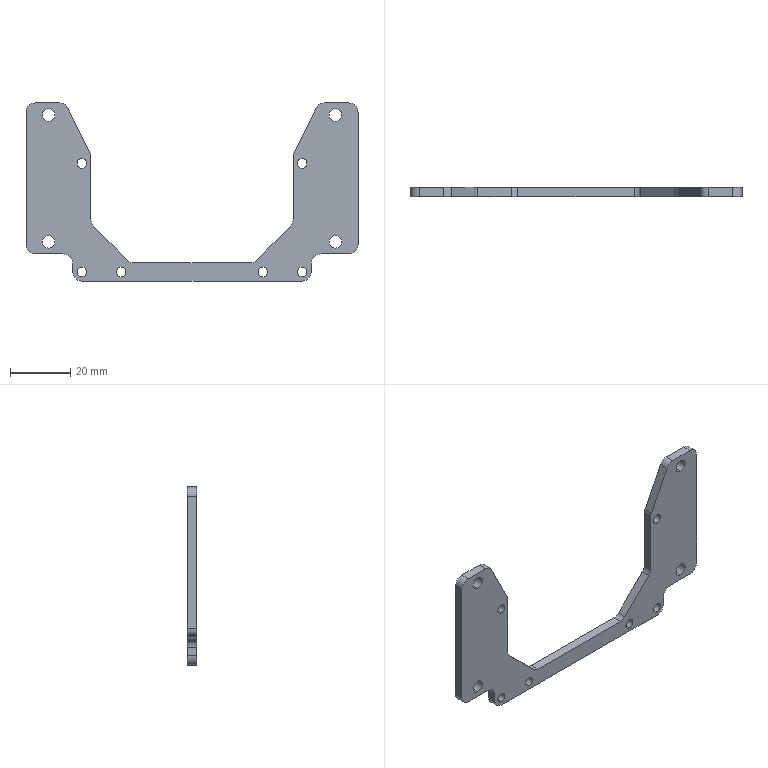Part | SolidWorks | features Chamfer 2, Extrusion 1, Fillet 1 | 1 solid | 62 faces | box 110 x 3 x 59 mm | volume 7718 mm3 | cylinder 40 | plane 22 | commonest cylinder face diameters 6 x20 3.2 x12 4.2 x8